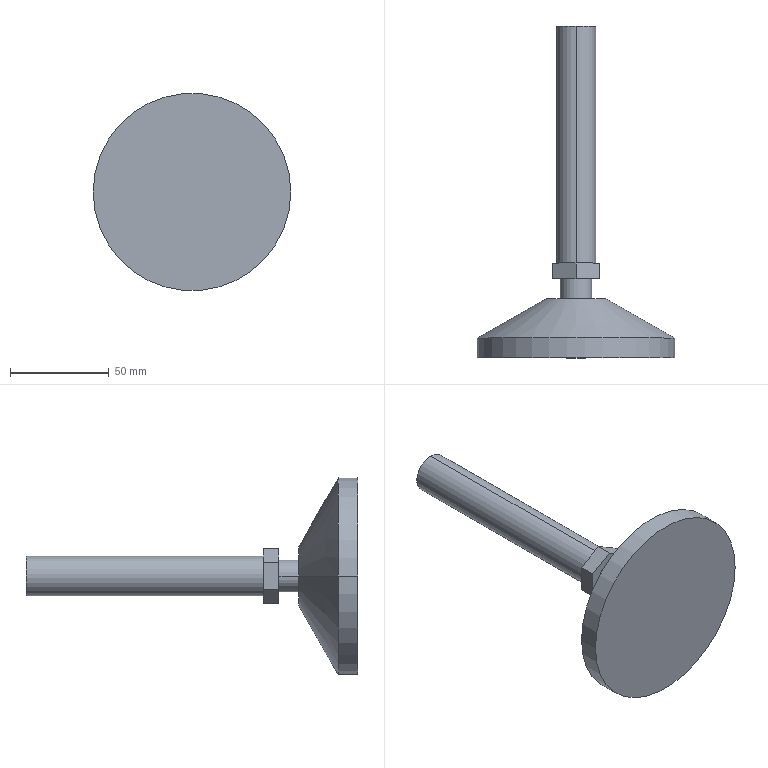Part | SolidWorks | features ICE 3, Revolution 1 | 1 solid | 19 faces | box 100 x 168 x 100 mm | volume 195020 mm3 | plane 11 | cylinder 6 | cone 2 | commonest cylinder face diameters 16 x2 20 x2 100 x2
STEP:
#1=CARTESIAN_POINT('',(0.,168.,10.));
#2=VERTEX_POINT('',#1);
#3=CARTESIAN_POINT('',(0.,168.,-10.));
#4=VERTEX_POINT('',#3);
#5=CARTESIAN_POINT('',(0.,168.,0.));
#6=DIRECTION('',(0.,1.,0.));
#7=DIRECTION('',(0.,0.,1.));
#8=AXIS2_PLACEMENT_3D('',#5,#6,#7);
#9=CIRCLE('',#8,10.);
#10=EDGE_CURVE('',#2,#4,#9,.T.);
#11=ORIENTED_EDGE('',*,*,#10,.F.);
#12=CARTESIAN_POINT('',(0.,48.,10.));
#13=VERTEX_POINT('',#12);
#14=CARTESIAN_POINT('',(0.,168.,10.));
#15=DIRECTION('',(0.,-1.,0.));
#16=VECTOR('',#15,1000.);
#17=LINE('',#14,#16);
#18=EDGE_CURVE('',#2,#13,#17,.T.);
#19=ORIENTED_EDGE('',*,*,#18,.T.);
#20=CARTESIAN_POINT('',(0.,48.,-10.));
#21=VERTEX_POINT('',#20);
#22=CARTESIAN_POINT('',(0.,48.,0.));
#23=DIRECTION('',(0.,1.,0.));
#24=DIRECTION('',(0.,0.,1.));
#25=AXIS2_PLACEMENT_3D('',#22,#23,#24);
#26=CIRCLE('',#25,10.);
#27=EDGE_CURVE('',#13,#21,#26,.T.);
#28=ORIENTED_EDGE('',*,*,#27,.T.);
#29=CARTESIAN_POINT('',(0.,168.,-10.));
#30=DIRECTION('',(0.,-1.,0.));
#31=VECTOR('',#30,1000.);
#32=LINE('',#29,#31);
#33=EDGE_CURVE('',#4,#21,#32,.T.);
#34=ORIENTED_EDGE('',*,*,#33,.F.);
#35=EDGE_LOOP('',(#11,#19,#28,#34));
#36=FACE_OUTER_BOUND('',#35,.T.);
#37=CARTESIAN_POINT('',(0.,168.,0.));
#38=DIRECTION('',(0.,-1.,0.));
#39=DIRECTION('',(0.,0.,-1.));
#40=AXIS2_PLACEMENT_3D('',#37,#38,#39);
#41=CYLINDRICAL_SURFACE('',#40,10.);
#42=ADVANCED_FACE('',(#36),#41,.T.);
#43=CARTESIAN_POINT('',(-8.,40.,0.));
#44=VERTEX_POINT('',#43);
#45=CARTESIAN_POINT('',(8.,40.,0.));
#46=VERTEX_POINT('',#45);
#47=CARTESIAN_POINT('',(0.,40.,0.));
#48=DIRECTION('',(0.,1.,0.));
#49=DIRECTION('',(-1.,0.,0.));
#50=AXIS2_PLACEMENT_3D('',#47,#48,#49);
#51=CIRCLE('',#50,8.);
#52=EDGE_CURVE('',#44,#46,#51,.T.);
#53=ORIENTED_EDGE('',*,*,#52,.F.);
#54=CARTESIAN_POINT('',(-8.,30.,0.));
#55=VERTEX_POINT('',#54);
#56=CARTESIAN_POINT('',(-8.,40.,0.));
#57=DIRECTION('',(0.,-1.,0.));
#58=VECTOR('',#57,1000.);
#59=LINE('',#56,#58);
#60=EDGE_CURVE('',#44,#55,#59,.T.);
#61=ORIENTED_EDGE('',*,*,#60,.T.);
#62=CARTESIAN_POINT('',(8.,30.,0.));
#63=VERTEX_POINT('',#62);
#64=CARTESIAN_POINT('',(0.,30.,0.));
#65=DIRECTION('',(0.,1.,0.));
#66=DIRECTION('',(1.,0.,0.));
#67=AXIS2_PLACEMENT_3D('',#64,#65,#66);
#68=CIRCLE('',#67,8.);
#69=EDGE_CURVE('',#55,#63,#68,.T.);
#70=ORIENTED_EDGE('',*,*,#69,.T.);
#71=CARTESIAN_POINT('',(8.,40.,0.));
#72=DIRECTION('',(0.,-1.,0.));
#73=VECTOR('',#72,1000.);
#74=LINE('',#71,#73);
#75=EDGE_CURVE('',#46,#63,#74,.T.);
#76=ORIENTED_EDGE('',*,*,#75,.F.);
#77=EDGE_LOOP('',(#53,#61,#70,#76));
#78=FACE_OUTER_BOUND('',#77,.T.);
#79=CARTESIAN_POINT('',(0.,40.,0.));
#80=DIRECTION('',(0.,-1.,0.));
#81=DIRECTION('',(1.,0.,0.));
#82=AXIS2_PLACEMENT_3D('',#79,#80,#81);
#83=CYLINDRICAL_SURFACE('',#82,8.);
#84=ADVANCED_FACE('',(#78),#83,.T.);
#85=CARTESIAN_POINT('',(-15.,30.,0.));
#86=VERTEX_POINT('',#85);
#87=CARTESIAN_POINT('',(15.,30.,0.));
#88=VERTEX_POINT('',#87);
#89=CARTESIAN_POINT('',(0.,30.,0.));
#90=DIRECTION('',(0.,1.,0.));
#91=DIRECTION('',(-1.,0.,0.));
#92=AXIS2_PLACEMENT_3D('',#89,#90,#91);
#93=CIRCLE('',#92,15.);
#94=EDGE_CURVE('',#86,#88,#93,.T.);
#95=ORIENTED_EDGE('',*,*,#94,.F.);
#96=CARTESIAN_POINT('',(-50.,10.,0.));
#97=VERTEX_POINT('',#96);
#98=CARTESIAN_POINT('',(-50.,10.,0.));
#99=DIRECTION('',(-0.8682,-0.4961,0.));
#100=VECTOR('',#99,1000.);
#101=LINE('',#98,#100);
#102=EDGE_CURVE('',#86,#97,#101,.T.);
#103=ORIENTED_EDGE('',*,*,#102,.T.);
#104=CARTESIAN_POINT('',(50.,10.,0.));
#105=VERTEX_POINT('',#104);
#106=CARTESIAN_POINT('',(0.,10.,0.));
#107=DIRECTION('',(0.,1.,0.));
#108=DIRECTION('',(-1.,0.,0.));
#109=AXIS2_PLACEMENT_3D('',#106,#107,#108);
#110=CIRCLE('',#109,50.);
#111=EDGE_CURVE('',#97,#105,#110,.T.);
#112=ORIENTED_EDGE('',*,*,#111,.T.);
#113=CARTESIAN_POINT('',(50.,10.,0.));
#114=DIRECTION('',(0.8682,-0.4961,0.));
#115=VECTOR('',#114,1000.);
#116=LINE('',#113,#115);
#117=EDGE_CURVE('',#88,#105,#116,.T.);
#118=ORIENTED_EDGE('',*,*,#117,.F.);
#119=EDGE_LOOP('',(#95,#103,#112,#118));
#120=FACE_OUTER_BOUND('',#119,.T.);
#121=CARTESIAN_POINT('',(0.,10.,0.));
#122=DIRECTION('',(0.,-1.,0.));
#123=DIRECTION('',(1.,0.,0.));
#124=AXIS2_PLACEMENT_3D('',#121,#122,#123);
#125=CONICAL_SURFACE('',#124,50.,1.052);
#126=ADVANCED_FACE('',(#120),#125,.T.);
#127=CARTESIAN_POINT('',(-50.,0.,0.));
#128=VERTEX_POINT('',#127);
#129=CARTESIAN_POINT('',(50.,0.,0.));
#130=VERTEX_POINT('',#129);
#131=CARTESIAN_POINT('',(0.,0.,0.));
#132=DIRECTION('',(0.,1.,0.));
#133=DIRECTION('',(-1.,0.,0.));
#134=AXIS2_PLACEMENT_3D('',#131,#132,#133);
#135=CIRCLE('',#134,50.);
#136=EDGE_CURVE('',#128,#130,#135,.T.);
#137=ORIENTED_EDGE('',*,*,#136,.T.);
#138=CARTESIAN_POINT('',(50.,30.,0.));
#139=DIRECTION('',(0.,1.,0.));
#140=VECTOR('',#139,1000.);
#141=LINE('',#138,#140);
#142=EDGE_CURVE('',#130,#105,#141,.T.);
#143=ORIENTED_EDGE('',*,*,#142,.T.);
#144=ORIENTED_EDGE('',*,*,#111,.F.);
#145=CARTESIAN_POINT('',(-50.,30.,0.));
#146=DIRECTION('',(0.,1.,0.));
#147=VECTOR('',#146,1000.);
#148=LINE('',#145,#147);
#149=EDGE_CURVE('',#128,#97,#148,.T.);
#150=ORIENTED_EDGE('',*,*,#149,.F.);
#151=EDGE_LOOP('',(#137,#143,#144,#150));
#152=FACE_OUTER_BOUND('',#151,.T.);
#153=CARTESIAN_POINT('',(0.,30.,0.));
#154=DIRECTION('',(0.,1.,0.));
#155=DIRECTION('',(-1.,0.,0.));
#156=AXIS2_PLACEMENT_3D('',#153,#154,#155);
#157=CYLINDRICAL_SURFACE('',#156,50.);
#158=ADVANCED_FACE('',(#152),#157,.T.);
#159=CARTESIAN_POINT('',(12.,48.,-6.928));
#160=VERTEX_POINT('',#159);
#161=CARTESIAN_POINT('',(0.,48.,-13.856));
#162=VERTEX_POINT('',#161);
#163=CARTESIAN_POINT('',(12.,48.,-6.928));
#164=DIRECTION('',(-0.866,0.,-0.5));
#165=VECTOR('',#164,1000.);
#166=LINE('',#163,#165);
#167=EDGE_CURVE('',#160,#162,#166,.T.);
#168=ORIENTED_EDGE('',*,*,#167,.T.);
#169=CARTESIAN_POINT('',(-12.,48.,-6.928));
#170=VERTEX_POINT('',#169);
#171=CARTESIAN_POINT('',(0.,48.,-13.856));
#172=DIRECTION('',(-0.866,0.,0.5));
#173=VECTOR('',#172,1000.);
#174=LINE('',#171,#173);
#175=EDGE_CURVE('',#162,#170,#174,.T.);
#176=ORIENTED_EDGE('',*,*,#175,.T.);
#177=CARTESIAN_POINT('',(-12.,48.,6.928));
#178=VERTEX_POINT('',#177);
#179=CARTESIAN_POINT('',(-12.,48.,-6.928));
#180=DIRECTION('',(0.,0.,1.));
#181=VECTOR('',#180,1000.);
#182=LINE('',#179,#181);
#183=EDGE_CURVE('',#170,#178,#182,.T.);
#184=ORIENTED_EDGE('',*,*,#183,.T.);
#185=CARTESIAN_POINT('',(0.,48.,13.856));
#186=VERTEX_POINT('',#185);
#187=CARTESIAN_POINT('',(-12.,48.,6.928));
#188=DIRECTION('',(0.866,0.,0.5));
#189=VECTOR('',#188,1000.);
#190=LINE('',#187,#189);
#191=EDGE_CURVE('',#178,#186,#190,.T.);
#192=ORIENTED_EDGE('',*,*,#191,.T.);
#193=CARTESIAN_POINT('',(12.,48.,6.928));
#194=VERTEX_POINT('',#193);
#195=CARTESIAN_POINT('',(0.,48.,13.856));
#196=DIRECTION('',(0.866,0.,-0.5));
#197=VECTOR('',#196,1000.);
#198=LINE('',#195,#197);
#199=EDGE_CURVE('',#186,#194,#198,.T.);
#200=ORIENTED_EDGE('',*,*,#199,.T.);
#201=CARTESIAN_POINT('',(12.,48.,6.928));
#202=DIRECTION('',(0.,0.,-1.));
#203=VECTOR('',#202,1000.);
#204=LINE('',#201,#203);
#205=EDGE_CURVE('',#194,#160,#204,.T.);
#206=ORIENTED_EDGE('',*,*,#205,.T.);
#207=EDGE_LOOP('',(#168,#176,#184,#192,#200,#206));
#208=FACE_OUTER_BOUND('',#207,.T.);
#209=CARTESIAN_POINT('',(0.,48.,0.));
#210=DIRECTION('',(0.,1.,0.));
#211=DIRECTION('',(0.,0.,1.));
#212=AXIS2_PLACEMENT_3D('',#209,#210,#211);
#213=CIRCLE('',#212,10.);
#214=EDGE_CURVE('',#21,#13,#213,.T.);
#215=ORIENTED_EDGE('',*,*,#214,.F.);
#216=ORIENTED_EDGE('',*,*,#27,.F.);
#217=EDGE_LOOP('',(#215,#216));
#218=FACE_BOUND('',#217,.T.);
#219=CARTESIAN_POINT('',(0.,48.,0.));
#220=DIRECTION('',(0.,1.,0.));
#221=DIRECTION('',(0.,0.,1.));
#222=AXIS2_PLACEMENT_3D('',#219,#220,#221);
#223=PLANE('',#222);
#224=ADVANCED_FACE('',(#208,#218),#223,.T.);
#225=CARTESIAN_POINT('',(0.,30.,0.));
#226=DIRECTION('',(0.,1.,0.));
#227=DIRECTION('',(-1.,0.,0.));
#228=AXIS2_PLACEMENT_3D('',#225,#226,#227);
#229=CIRCLE('',#228,15.);
#230=EDGE_CURVE('',#88,#86,#229,.T.);
#231=ORIENTED_EDGE('',*,*,#230,.T.);
#232=ORIENTED_EDGE('',*,*,#94,.T.);
#233=EDGE_LOOP('',(#231,#232));
#234=FACE_OUTER_BOUND('',#233,.T.);
#235=CARTESIAN_POINT('',(0.,30.,0.));
#236=DIRECTION('',(0.,1.,0.));
#237=DIRECTION('',(1.,0.,0.));
#238=AXIS2_PLACEMENT_3D('',#235,#236,#237);
#239=CIRCLE('',#238,8.);
#240=EDGE_CURVE('',#63,#55,#239,.T.);
#241=ORIENTED_EDGE('',*,*,#240,.F.);
#242=ORIENTED_EDGE('',*,*,#69,.F.);
#243=EDGE_LOOP('',(#241,#242));
#244=FACE_BOUND('',#243,.T.);
#245=CARTESIAN_POINT('',(15.,30.,0.));
#246=DIRECTION('',(0.,-1.,0.));
#247=DIRECTION('',(1.,0.,0.));
#248=AXIS2_PLACEMENT_3D('',#245,#246,#247);
#249=PLANE('',#248);
#250=ADVANCED_FACE('',(#234,#244),#249,.F.);
#251=ORIENTED_EDGE('',*,*,#136,.F.);
#252=CARTESIAN_POINT('',(0.,0.,0.));
#253=DIRECTION('',(0.,1.,0.));
#254=DIRECTION('',(-1.,0.,0.));
#255=AXIS2_PLACEMENT_3D('',#252,#253,#254);
#256=CIRCLE('',#255,50.);
#257=EDGE_CURVE('',#130,#128,#256,.T.);
#258=ORIENTED_EDGE('',*,*,#257,.F.);
#259=EDGE_LOOP('',(#251,#258));
#260=FACE_OUTER_BOUND('',#259,.T.);
#261=CARTESIAN_POINT('',(0.,0.,0.));
#262=DIRECTION('',(0.,1.,0.));
#263=DIRECTION('',(-1.,0.,0.));
#264=AXIS2_PLACEMENT_3D('',#261,#262,#263);
#265=PLANE('',#264);
#266=ADVANCED_FACE('',(#260),#265,.F.);
#267=ORIENTED_EDGE('',*,*,#142,.F.);
#268=ORIENTED_EDGE('',*,*,#257,.T.);
#269=ORIENTED_EDGE('',*,*,#149,.T.);
#270=CARTESIAN_POINT('',(0.,10.,0.));
#271=DIRECTION('',(0.,1.,0.));
#272=DIRECTION('',(-1.,0.,0.));
#273=AXIS2_PLACEMENT_3D('',#270,#271,#272);
#274=CIRCLE('',#273,50.);
#275=EDGE_CURVE('',#105,#97,#274,.T.);
#276=ORIENTED_EDGE('',*,*,#275,.F.);
#277=EDGE_LOOP('',(#267,#268,#269,#276));
#278=FACE_OUTER_BOUND('',#277,.T.);
#279=CARTESIAN_POINT('',(0.,30.,0.));
#280=DIRECTION('',(0.,1.,0.));
#281=DIRECTION('',(-1.,0.,0.));
#282=AXIS2_PLACEMENT_3D('',#279,#280,#281);
#283=CYLINDRICAL_SURFACE('',#282,50.);
#284=ADVANCED_FACE('',(#278),#283,.T.);
#285=ORIENTED_EDGE('',*,*,#102,.F.);
#286=ORIENTED_EDGE('',*,*,#230,.F.);
#287=ORIENTED_EDGE('',*,*,#117,.T.);
#288=ORIENTED_EDGE('',*,*,#275,.T.);
#289=EDGE_LOOP('',(#285,#286,#287,#288));
#290=FACE_OUTER_BOUND('',#289,.T.);
#291=CARTESIAN_POINT('',(0.,10.,0.));
#292=DIRECTION('',(0.,-1.,0.));
#293=DIRECTION('',(1.,0.,0.));
#294=AXIS2_PLACEMENT_3D('',#291,#292,#293);
#295=CONICAL_SURFACE('',#294,50.,1.052);
#296=ADVANCED_FACE('',(#290),#295,.T.);
#297=ORIENTED_EDGE('',*,*,#60,.F.);
#298=CARTESIAN_POINT('',(0.,40.,0.));
#299=DIRECTION('',(0.,1.,0.));
#300=DIRECTION('',(-1.,0.,0.));
#301=AXIS2_PLACEMENT_3D('',#298,#299,#300);
#302=CIRCLE('',#301,8.);
#303=EDGE_CURVE('',#46,#44,#302,.T.);
#304=ORIENTED_EDGE('',*,*,#303,.F.);
#305=ORIENTED_EDGE('',*,*,#75,.T.);
#306=ORIENTED_EDGE('',*,*,#240,.T.);
#307=EDGE_LOOP('',(#297,#304,#305,#306));
#308=FACE_OUTER_BOUND('',#307,.T.);
#309=CARTESIAN_POINT('',(0.,40.,0.));
#310=DIRECTION('',(0.,-1.,0.));
#311=DIRECTION('',(1.,0.,0.));
#312=AXIS2_PLACEMENT_3D('',#309,#310,#311);
#313=CYLINDRICAL_SURFACE('',#312,8.);
#314=ADVANCED_FACE('',(#308),#313,.T.);
#315=CARTESIAN_POINT('',(12.,40.,-6.928));
#316=VERTEX_POINT('',#315);
#317=CARTESIAN_POINT('',(0.,40.,-13.856));
#318=VERTEX_POINT('',#317);
#319=CARTESIAN_POINT('',(12.,40.,-6.928));
#320=DIRECTION('',(-0.866,0.,-0.5));
#321=VECTOR('',#320,1000.);
#322=LINE('',#319,#321);
#323=EDGE_CURVE('',#316,#318,#322,.T.);
#324=ORIENTED_EDGE('',*,*,#323,.F.);
#325=CARTESIAN_POINT('',(12.,40.,6.928));
#326=VERTEX_POINT('',#325);
#327=CARTESIAN_POINT('',(12.,40.,6.928));
#328=DIRECTION('',(0.,0.,-1.));
#329=VECTOR('',#328,1000.);
#330=LINE('',#327,#329);
#331=EDGE_CURVE('',#326,#316,#330,.T.);
#332=ORIENTED_EDGE('',*,*,#331,.F.);
#333=CARTESIAN_POINT('',(0.,40.,13.856));
#334=VERTEX_POINT('',#333);
#335=CARTESIAN_POINT('',(0.,40.,13.856));
#336=DIRECTION('',(0.866,0.,-0.5));
#337=VECTOR('',#336,1000.);
#338=LINE('',#335,#337);
#339=EDGE_CURVE('',#334,#326,#338,.T.);
#340=ORIENTED_EDGE('',*,*,#339,.F.);
#341=CARTESIAN_POINT('',(-12.,40.,6.928));
#342=VERTEX_POINT('',#341);
#343=CARTESIAN_POINT('',(-12.,40.,6.928));
#344=DIRECTION('',(0.866,0.,0.5));
#345=VECTOR('',#344,1000.);
#346=LINE('',#343,#345);
#347=EDGE_CURVE('',#342,#334,#346,.T.);
#348=ORIENTED_EDGE('',*,*,#347,.F.);
#349=CARTESIAN_POINT('',(-12.,40.,-6.928));
#350=VERTEX_POINT('',#349);
#351=CARTESIAN_POINT('',(-12.,40.,-6.928));
#352=DIRECTION('',(0.,0.,1.));
#353=VECTOR('',#352,1000.);
#354=LINE('',#351,#353);
#355=EDGE_CURVE('',#350,#342,#354,.T.);
#356=ORIENTED_EDGE('',*,*,#355,.F.);
#357=CARTESIAN_POINT('',(0.,40.,-13.856));
#358=DIRECTION('',(-0.866,0.,0.5));
#359=VECTOR('',#358,1000.);
#360=LINE('',#357,#359);
#361=EDGE_CURVE('',#318,#350,#360,.T.);
#362=ORIENTED_EDGE('',*,*,#361,.F.);
#363=EDGE_LOOP('',(#324,#332,#340,#348,#356,#362));
#364=FACE_OUTER_BOUND('',#363,.T.);
#365=ORIENTED_EDGE('',*,*,#303,.T.);
#366=ORIENTED_EDGE('',*,*,#52,.T.);
#367=EDGE_LOOP('',(#365,#366));
#368=FACE_BOUND('',#367,.T.);
#369=CARTESIAN_POINT('',(0.,40.,0.));
#370=DIRECTION('',(0.,1.,0.));
#371=DIRECTION('',(0.,0.,1.));
#372=AXIS2_PLACEMENT_3D('',#369,#370,#371);
#373=PLANE('',#372);
#374=ADVANCED_FACE('',(#364,#368),#373,.F.);
#375=ORIENTED_EDGE('',*,*,#323,.T.);
#376=CARTESIAN_POINT('',(0.,48.,-13.856));
#377=DIRECTION('',(0.,-1.,0.));
#378=VECTOR('',#377,1000.);
#379=LINE('',#376,#378);
#380=EDGE_CURVE('',#162,#318,#379,.T.);
#381=ORIENTED_EDGE('',*,*,#380,.F.);
#382=ORIENTED_EDGE('',*,*,#167,.F.);
#383=CARTESIAN_POINT('',(12.,48.,-6.928));
#384=DIRECTION('',(0.,-1.,0.));
#385=VECTOR('',#384,1000.);
#386=LINE('',#383,#385);
#387=EDGE_CURVE('',#160,#316,#386,.T.);
#388=ORIENTED_EDGE('',*,*,#387,.T.);
#389=EDGE_LOOP('',(#375,#381,#382,#388));
#390=FACE_OUTER_BOUND('',#389,.T.);
#391=CARTESIAN_POINT('',(12.,48.,-6.928));
#392=DIRECTION('',(-0.5,0.,0.866));
#393=DIRECTION('',(0.866,0.,0.5));
#394=AXIS2_PLACEMENT_3D('',#391,#392,#393);
#395=PLANE('',#394);
#396=ADVANCED_FACE('',(#390),#395,.F.);
#397=ORIENTED_EDGE('',*,*,#361,.T.);
#398=CARTESIAN_POINT('',(-12.,48.,-6.928));
#399=DIRECTION('',(0.,-1.,0.));
#400=VECTOR('',#399,1000.);
#401=LINE('',#398,#400);
#402=EDGE_CURVE('',#170,#350,#401,.T.);
#403=ORIENTED_EDGE('',*,*,#402,.F.);
#404=ORIENTED_EDGE('',*,*,#175,.F.);
#405=ORIENTED_EDGE('',*,*,#380,.T.);
#406=EDGE_LOOP('',(#397,#403,#404,#405));
#407=FACE_OUTER_BOUND('',#406,.T.);
#408=CARTESIAN_POINT('',(0.,48.,-13.856));
#409=DIRECTION('',(0.5,0.,0.866));
#410=DIRECTION('',(0.866,0.,-0.5));
#411=AXIS2_PLACEMENT_3D('',#408,#409,#410);
#412=PLANE('',#411);
#413=ADVANCED_FACE('',(#407),#412,.F.);
#414=ORIENTED_EDGE('',*,*,#355,.T.);
#415=CARTESIAN_POINT('',(-12.,48.,6.928));
#416=DIRECTION('',(0.,-1.,0.));
#417=VECTOR('',#416,1000.);
#418=LINE('',#415,#417);
#419=EDGE_CURVE('',#178,#342,#418,.T.);
#420=ORIENTED_EDGE('',*,*,#419,.F.);
#421=ORIENTED_EDGE('',*,*,#183,.F.);
#422=ORIENTED_EDGE('',*,*,#402,.T.);
#423=EDGE_LOOP('',(#414,#420,#421,#422));
#424=FACE_OUTER_BOUND('',#423,.T.);
#425=CARTESIAN_POINT('',(-12.,48.,-6.928));
#426=DIRECTION('',(1.,0.,0.));
#427=DIRECTION('',(0.,0.,-1.));
#428=AXIS2_PLACEMENT_3D('',#425,#426,#427);
#429=PLANE('',#428);
#430=ADVANCED_FACE('',(#424),#429,.F.);
#431=ORIENTED_EDGE('',*,*,#347,.T.);
#432=CARTESIAN_POINT('',(0.,48.,13.856));
#433=DIRECTION('',(0.,-1.,0.));
#434=VECTOR('',#433,1000.);
#435=LINE('',#432,#434);
#436=EDGE_CURVE('',#186,#334,#435,.T.);
#437=ORIENTED_EDGE('',*,*,#436,.F.);
#438=ORIENTED_EDGE('',*,*,#191,.F.);
#439=ORIENTED_EDGE('',*,*,#419,.T.);
#440=EDGE_LOOP('',(#431,#437,#438,#439));
#441=FACE_OUTER_BOUND('',#440,.T.);
#442=CARTESIAN_POINT('',(-12.,48.,6.928));
#443=DIRECTION('',(0.5,0.,-0.866));
#444=DIRECTION('',(-0.866,0.,-0.5));
#445=AXIS2_PLACEMENT_3D('',#442,#443,#444);
#446=PLANE('',#445);
#447=ADVANCED_FACE('',(#441),#446,.F.);
#448=ORIENTED_EDGE('',*,*,#339,.T.);
#449=CARTESIAN_POINT('',(12.,48.,6.928));
#450=DIRECTION('',(0.,-1.,0.));
#451=VECTOR('',#450,1000.);
#452=LINE('',#449,#451);
#453=EDGE_CURVE('',#194,#326,#452,.T.);
#454=ORIENTED_EDGE('',*,*,#453,.F.);
#455=ORIENTED_EDGE('',*,*,#199,.F.);
#456=ORIENTED_EDGE('',*,*,#436,.T.);
#457=EDGE_LOOP('',(#448,#454,#455,#456));
#458=FACE_OUTER_BOUND('',#457,.T.);
#459=CARTESIAN_POINT('',(0.,48.,13.856));
#460=DIRECTION('',(-0.5,0.,-0.866));
#461=DIRECTION('',(-0.866,0.,0.5));
#462=AXIS2_PLACEMENT_3D('',#459,#460,#461);
#463=PLANE('',#462);
#464=ADVANCED_FACE('',(#458),#463,.F.);
#465=ORIENTED_EDGE('',*,*,#331,.T.);
#466=ORIENTED_EDGE('',*,*,#387,.F.);
#467=ORIENTED_EDGE('',*,*,#205,.F.);
#468=ORIENTED_EDGE('',*,*,#453,.T.);
#469=EDGE_LOOP('',(#465,#466,#467,#468));
#470=FACE_OUTER_BOUND('',#469,.T.);
#471=CARTESIAN_POINT('',(12.,48.,6.928));
#472=DIRECTION('',(-1.,0.,0.));
#473=DIRECTION('',(0.,0.,1.));
#474=AXIS2_PLACEMENT_3D('',#471,#472,#473);
#475=PLANE('',#474);
#476=ADVANCED_FACE('',(#470),#475,.F.);
#477=ORIENTED_EDGE('',*,*,#18,.F.);
#478=CARTESIAN_POINT('',(0.,168.,0.));
#479=DIRECTION('',(0.,1.,0.));
#480=DIRECTION('',(0.,0.,1.));
#481=AXIS2_PLACEMENT_3D('',#478,#479,#480);
#482=CIRCLE('',#481,10.);
#483=EDGE_CURVE('',#4,#2,#482,.T.);
#484=ORIENTED_EDGE('',*,*,#483,.F.);
#485=ORIENTED_EDGE('',*,*,#33,.T.);
#486=ORIENTED_EDGE('',*,*,#214,.T.);
#487=EDGE_LOOP('',(#477,#484,#485,#486));
#488=FACE_OUTER_BOUND('',#487,.T.);
#489=CARTESIAN_POINT('',(0.,168.,0.));
#490=DIRECTION('',(0.,-1.,0.));
#491=DIRECTION('',(0.,0.,-1.));
#492=AXIS2_PLACEMENT_3D('',#489,#490,#491);
#493=CYLINDRICAL_SURFACE('',#492,10.);
#494=ADVANCED_FACE('',(#488),#493,.T.);
#495=ORIENTED_EDGE('',*,*,#483,.T.);
#496=ORIENTED_EDGE('',*,*,#10,.T.);
#497=EDGE_LOOP('',(#495,#496));
#498=FACE_OUTER_BOUND('',#497,.T.);
#499=CARTESIAN_POINT('',(0.,168.,0.));
#500=DIRECTION('',(0.,1.,0.));
#501=DIRECTION('',(0.,0.,1.));
#502=AXIS2_PLACEMENT_3D('',#499,#500,#501);
#503=PLANE('',#502);
#504=ADVANCED_FACE('',(#498),#503,.T.);
#505=CLOSED_SHELL('',(#42,#84,#126,#158,#224,#250,#266,#284,#296,#314,#374,#396,#413,#430,#447,#464,#476,#494,#504));
#506=MANIFOLD_SOLID_BREP('',#505);
#507=CARTESIAN_POINT('',(0.,0.,0.));
#508=DIRECTION('',(0.,0.,1.));
#509=DIRECTION('',(1.,0.,0.));
#510=AXIS2_PLACEMENT_3D('',#507,#508,#509);
#511=(LENGTH_UNIT()NAMED_UNIT(*)SI_UNIT(.MILLI.,.METRE.));
#512=UNCERTAINTY_MEASURE_WITH_UNIT(LENGTH_MEASURE(0.00001),#511,'','');
#513=(NAMED_UNIT(*)PLANE_ANGLE_UNIT()SI_UNIT($,.RADIAN.));
#514=(NAMED_UNIT(*)SI_UNIT($,.STERADIAN.)SOLID_ANGLE_UNIT());
#515=(GEOMETRIC_REPRESENTATION_CONTEXT(3)GLOBAL_UNCERTAINTY_ASSIGNED_CONTEXT((#512))GLOBAL_UNIT_ASSIGNED_CONTEXT((#511,#513,#514))REPRESENTATION_CONTEXT('',''));
#516=ADVANCED_BREP_SHAPE_REPRESENTATION('',(#506,#510),#515);